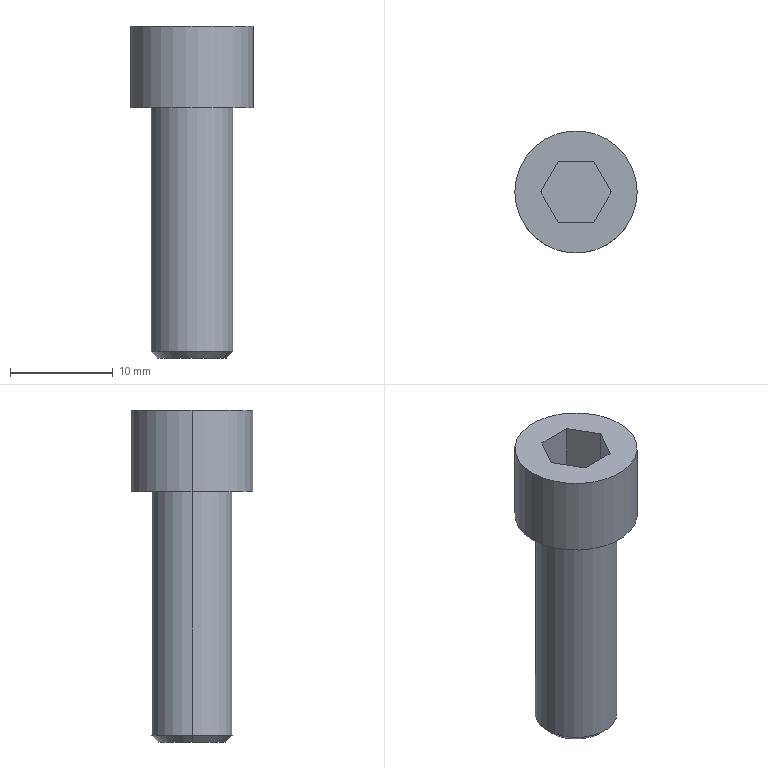Part | STEP file | 4-20.sldasm-Part-427 | 1 solid | 16 faces | box 11.91 x 11.91 x 32.34 mm | volume 1927 mm3 | plane 10 | cylinder 4 | cone 2 | commonest cylinder face diameters 7.94 x2 11.91 x2
STEP:
#1=CARTESIAN_POINT('',(-3.325,-75.,288.982));
#2=VERTEX_POINT('',#1);
#3=CARTESIAN_POINT('',(3.325,-75.,288.982));
#4=VERTEX_POINT('',#3);
#5=CARTESIAN_POINT('',(0.,-75.,288.982));
#6=DIRECTION('',(0.,0.,-1.));
#7=DIRECTION('',(1.,0.,0.));
#8=AXIS2_PLACEMENT_3D('',#5,#6,#7);
#9=CIRCLE('',#8,3.325);
#10=EDGE_CURVE('',#2,#4,#9,.T.);
#11=ORIENTED_EDGE('',*,*,#10,.F.);
#12=CARTESIAN_POINT('',(-3.97,-75.,289.627));
#13=VERTEX_POINT('',#12);
#14=CARTESIAN_POINT('',(-3.97,-75.,289.627));
#15=DIRECTION('',(-0.7071,0.,0.7071));
#16=VECTOR('',#15,1000.);
#17=LINE('',#14,#16);
#18=EDGE_CURVE('',#2,#13,#17,.T.);
#19=ORIENTED_EDGE('',*,*,#18,.T.);
#20=CARTESIAN_POINT('',(3.97,-75.,289.627));
#21=VERTEX_POINT('',#20);
#22=CARTESIAN_POINT('',(0.,-75.,289.627));
#23=DIRECTION('',(0.,0.,1.));
#24=DIRECTION('',(1.,0.,0.));
#25=AXIS2_PLACEMENT_3D('',#22,#23,#24);
#26=CIRCLE('',#25,3.97);
#27=EDGE_CURVE('',#21,#13,#26,.T.);
#28=ORIENTED_EDGE('',*,*,#27,.F.);
#29=CARTESIAN_POINT('',(3.97,-75.,289.627));
#30=DIRECTION('',(0.7071,0.,0.7071));
#31=VECTOR('',#30,1000.);
#32=LINE('',#29,#31);
#33=EDGE_CURVE('',#4,#21,#32,.T.);
#34=ORIENTED_EDGE('',*,*,#33,.F.);
#35=EDGE_LOOP('',(#11,#19,#28,#34));
#36=FACE_OUTER_BOUND('',#35,.T.);
#37=CARTESIAN_POINT('',(0.,-75.,289.627));
#38=DIRECTION('',(0.,0.,1.));
#39=DIRECTION('',(1.,0.,0.));
#40=AXIS2_PLACEMENT_3D('',#37,#38,#39);
#41=CONICAL_SURFACE('',#40,3.97,0.7854);
#42=ADVANCED_FACE('',(#36),#41,.T.);
#43=CARTESIAN_POINT('',(5.955,-75.,313.382));
#44=VERTEX_POINT('',#43);
#45=CARTESIAN_POINT('',(-5.955,-75.,313.382));
#46=VERTEX_POINT('',#45);
#47=CARTESIAN_POINT('',(0.,-75.,313.382));
#48=DIRECTION('',(0.,0.,1.));
#49=DIRECTION('',(1.,0.,0.));
#50=AXIS2_PLACEMENT_3D('',#47,#48,#49);
#51=CIRCLE('',#50,5.955);
#52=EDGE_CURVE('',#44,#46,#51,.T.);
#53=ORIENTED_EDGE('',*,*,#52,.T.);
#54=CARTESIAN_POINT('',(-5.955,-75.,321.322));
#55=VERTEX_POINT('',#54);
#56=CARTESIAN_POINT('',(-5.955,-75.,313.382));
#57=DIRECTION('',(0.,0.,1.));
#58=VECTOR('',#57,1000.);
#59=LINE('',#56,#58);
#60=EDGE_CURVE('',#46,#55,#59,.T.);
#61=ORIENTED_EDGE('',*,*,#60,.T.);
#62=CARTESIAN_POINT('',(5.955,-75.,321.322));
#63=VERTEX_POINT('',#62);
#64=CARTESIAN_POINT('',(0.,-75.,321.322));
#65=DIRECTION('',(0.,0.,1.));
#66=DIRECTION('',(1.,0.,0.));
#67=AXIS2_PLACEMENT_3D('',#64,#65,#66);
#68=CIRCLE('',#67,5.955);
#69=EDGE_CURVE('',#63,#55,#68,.T.);
#70=ORIENTED_EDGE('',*,*,#69,.F.);
#71=CARTESIAN_POINT('',(5.955,-75.,313.382));
#72=DIRECTION('',(0.,0.,1.));
#73=VECTOR('',#72,1000.);
#74=LINE('',#71,#73);
#75=EDGE_CURVE('',#44,#63,#74,.T.);
#76=ORIENTED_EDGE('',*,*,#75,.F.);
#77=EDGE_LOOP('',(#53,#61,#70,#76));
#78=FACE_OUTER_BOUND('',#77,.T.);
#79=CARTESIAN_POINT('',(0.,-75.,313.382));
#80=DIRECTION('',(0.,0.,1.));
#81=DIRECTION('',(1.,0.,0.));
#82=AXIS2_PLACEMENT_3D('',#79,#80,#81);
#83=CYLINDRICAL_SURFACE('',#82,5.955);
#84=ADVANCED_FACE('',(#78),#83,.T.);
#85=CARTESIAN_POINT('',(3.97,-75.,313.382));
#86=VERTEX_POINT('',#85);
#87=CARTESIAN_POINT('',(-3.97,-75.,313.382));
#88=VERTEX_POINT('',#87);
#89=CARTESIAN_POINT('',(0.,-75.,313.382));
#90=DIRECTION('',(0.,0.,1.));
#91=DIRECTION('',(1.,0.,0.));
#92=AXIS2_PLACEMENT_3D('',#89,#90,#91);
#93=CIRCLE('',#92,3.97);
#94=EDGE_CURVE('',#86,#88,#93,.T.);
#95=ORIENTED_EDGE('',*,*,#94,.F.);
#96=CARTESIAN_POINT('',(3.97,-75.,313.382));
#97=DIRECTION('',(0.,0.,-1.));
#98=VECTOR('',#97,1000.);
#99=LINE('',#96,#98);
#100=EDGE_CURVE('',#86,#21,#99,.T.);
#101=ORIENTED_EDGE('',*,*,#100,.T.);
#102=ORIENTED_EDGE('',*,*,#27,.T.);
#103=CARTESIAN_POINT('',(-3.97,-75.,313.382));
#104=DIRECTION('',(0.,0.,-1.));
#105=VECTOR('',#104,1000.);
#106=LINE('',#103,#105);
#107=EDGE_CURVE('',#88,#13,#106,.T.);
#108=ORIENTED_EDGE('',*,*,#107,.F.);
#109=EDGE_LOOP('',(#95,#101,#102,#108));
#110=FACE_OUTER_BOUND('',#109,.T.);
#111=CARTESIAN_POINT('',(0.,-75.,313.382));
#112=DIRECTION('',(0.,0.,-1.));
#113=DIRECTION('',(-1.,0.,0.));
#114=AXIS2_PLACEMENT_3D('',#111,#112,#113);
#115=CYLINDRICAL_SURFACE('',#114,3.97);
#116=ADVANCED_FACE('',(#110),#115,.T.);
#117=ORIENTED_EDGE('',*,*,#100,.F.);
#118=CARTESIAN_POINT('',(0.,-75.,313.382));
#119=DIRECTION('',(0.,0.,1.));
#120=DIRECTION('',(1.,0.,0.));
#121=AXIS2_PLACEMENT_3D('',#118,#119,#120);
#122=CIRCLE('',#121,3.97);
#123=EDGE_CURVE('',#88,#86,#122,.T.);
#124=ORIENTED_EDGE('',*,*,#123,.F.);
#125=ORIENTED_EDGE('',*,*,#107,.T.);
#126=CARTESIAN_POINT('',(0.,-75.,289.627));
#127=DIRECTION('',(0.,0.,1.));
#128=DIRECTION('',(1.,0.,0.));
#129=AXIS2_PLACEMENT_3D('',#126,#127,#128);
#130=CIRCLE('',#129,3.97);
#131=EDGE_CURVE('',#13,#21,#130,.T.);
#132=ORIENTED_EDGE('',*,*,#131,.T.);
#133=EDGE_LOOP('',(#117,#124,#125,#132));
#134=FACE_OUTER_BOUND('',#133,.T.);
#135=CARTESIAN_POINT('',(0.,-75.,313.382));
#136=DIRECTION('',(0.,0.,-1.));
#137=DIRECTION('',(-1.,0.,0.));
#138=AXIS2_PLACEMENT_3D('',#135,#136,#137);
#139=CYLINDRICAL_SURFACE('',#138,3.97);
#140=ADVANCED_FACE('',(#134),#139,.T.);
#141=CARTESIAN_POINT('',(0.,-75.,288.982));
#142=DIRECTION('',(0.,0.,-1.));
#143=DIRECTION('',(1.,0.,0.));
#144=AXIS2_PLACEMENT_3D('',#141,#142,#143);
#145=CIRCLE('',#144,3.325);
#146=EDGE_CURVE('',#4,#2,#145,.T.);
#147=ORIENTED_EDGE('',*,*,#146,.T.);
#148=ORIENTED_EDGE('',*,*,#10,.T.);
#149=EDGE_LOOP('',(#147,#148));
#150=FACE_OUTER_BOUND('',#149,.T.);
#151=CARTESIAN_POINT('',(0.,-75.,288.982));
#152=DIRECTION('',(0.,0.,1.));
#153=DIRECTION('',(1.,0.,0.));
#154=AXIS2_PLACEMENT_3D('',#151,#152,#153);
#155=PLANE('',#154);
#156=ADVANCED_FACE('',(#150),#155,.F.);
#157=ORIENTED_EDGE('',*,*,#52,.F.);
#158=CARTESIAN_POINT('',(0.,-75.,313.382));
#159=DIRECTION('',(0.,0.,1.));
#160=DIRECTION('',(1.,0.,0.));
#161=AXIS2_PLACEMENT_3D('',#158,#159,#160);
#162=CIRCLE('',#161,5.955);
#163=EDGE_CURVE('',#46,#44,#162,.T.);
#164=ORIENTED_EDGE('',*,*,#163,.F.);
#165=EDGE_LOOP('',(#157,#164));
#166=FACE_OUTER_BOUND('',#165,.T.);
#167=ORIENTED_EDGE('',*,*,#123,.T.);
#168=ORIENTED_EDGE('',*,*,#94,.T.);
#169=EDGE_LOOP('',(#167,#168));
#170=FACE_BOUND('',#169,.T.);
#171=CARTESIAN_POINT('',(0.,-75.,313.382));
#172=DIRECTION('',(0.,0.,-1.));
#173=DIRECTION('',(-1.,0.,0.));
#174=AXIS2_PLACEMENT_3D('',#171,#172,#173);
#175=PLANE('',#174);
#176=ADVANCED_FACE('',(#166,#170),#175,.T.);
#177=CARTESIAN_POINT('',(-1.719,-77.977,321.322));
#178=VERTEX_POINT('',#177);
#179=CARTESIAN_POINT('',(1.719,-77.977,321.322));
#180=VERTEX_POINT('',#179);
#181=CARTESIAN_POINT('',(-1.719,-77.977,321.322));
#182=DIRECTION('',(1.,0.,0.));
#183=VECTOR('',#182,1000.);
#184=LINE('',#181,#183);
#185=EDGE_CURVE('',#178,#180,#184,.T.);
#186=ORIENTED_EDGE('',*,*,#185,.F.);
#187=CARTESIAN_POINT('',(-3.438,-75.,321.322));
#188=VERTEX_POINT('',#187);
#189=CARTESIAN_POINT('',(-3.438,-75.,321.322));
#190=DIRECTION('',(0.5,-0.866,0.));
#191=VECTOR('',#190,1000.);
#192=LINE('',#189,#191);
#193=EDGE_CURVE('',#188,#178,#192,.T.);
#194=ORIENTED_EDGE('',*,*,#193,.F.);
#195=CARTESIAN_POINT('',(-1.719,-72.022,321.322));
#196=VERTEX_POINT('',#195);
#197=CARTESIAN_POINT('',(-1.719,-72.022,321.322));
#198=DIRECTION('',(-0.5,-0.866,0.));
#199=VECTOR('',#198,1000.);
#200=LINE('',#197,#199);
#201=EDGE_CURVE('',#196,#188,#200,.T.);
#202=ORIENTED_EDGE('',*,*,#201,.F.);
#203=CARTESIAN_POINT('',(1.719,-72.022,321.322));
#204=VERTEX_POINT('',#203);
#205=CARTESIAN_POINT('',(1.719,-72.022,321.322));
#206=DIRECTION('',(-1.,0.,0.));
#207=VECTOR('',#206,1000.);
#208=LINE('',#205,#207);
#209=EDGE_CURVE('',#204,#196,#208,.T.);
#210=ORIENTED_EDGE('',*,*,#209,.F.);
#211=CARTESIAN_POINT('',(3.438,-75.,321.322));
#212=VERTEX_POINT('',#211);
#213=CARTESIAN_POINT('',(3.438,-75.,321.322));
#214=DIRECTION('',(-0.5,0.866,0.));
#215=VECTOR('',#214,1000.);
#216=LINE('',#213,#215);
#217=EDGE_CURVE('',#212,#204,#216,.T.);
#218=ORIENTED_EDGE('',*,*,#217,.F.);
#219=CARTESIAN_POINT('',(1.719,-77.977,321.322));
#220=DIRECTION('',(0.5,0.866,0.));
#221=VECTOR('',#220,1000.);
#222=LINE('',#219,#221);
#223=EDGE_CURVE('',#180,#212,#222,.T.);
#224=ORIENTED_EDGE('',*,*,#223,.F.);
#225=EDGE_LOOP('',(#186,#194,#202,#210,#218,#224));
#226=FACE_BOUND('',#225,.T.);
#227=ORIENTED_EDGE('',*,*,#69,.T.);
#228=CARTESIAN_POINT('',(0.,-75.,321.322));
#229=DIRECTION('',(0.,0.,1.));
#230=DIRECTION('',(1.,0.,0.));
#231=AXIS2_PLACEMENT_3D('',#228,#229,#230);
#232=CIRCLE('',#231,5.955);
#233=EDGE_CURVE('',#55,#63,#232,.T.);
#234=ORIENTED_EDGE('',*,*,#233,.T.);
#235=EDGE_LOOP('',(#227,#234));
#236=FACE_OUTER_BOUND('',#235,.T.);
#237=CARTESIAN_POINT('',(0.,-75.,321.322));
#238=DIRECTION('',(0.,0.,1.));
#239=DIRECTION('',(1.,0.,0.));
#240=AXIS2_PLACEMENT_3D('',#237,#238,#239);
#241=PLANE('',#240);
#242=ADVANCED_FACE('',(#226,#236),#241,.T.);
#243=ORIENTED_EDGE('',*,*,#60,.F.);
#244=ORIENTED_EDGE('',*,*,#163,.T.);
#245=ORIENTED_EDGE('',*,*,#75,.T.);
#246=ORIENTED_EDGE('',*,*,#233,.F.);
#247=EDGE_LOOP('',(#243,#244,#245,#246));
#248=FACE_OUTER_BOUND('',#247,.T.);
#249=CARTESIAN_POINT('',(0.,-75.,313.382));
#250=DIRECTION('',(0.,0.,1.));
#251=DIRECTION('',(1.,0.,0.));
#252=AXIS2_PLACEMENT_3D('',#249,#250,#251);
#253=CYLINDRICAL_SURFACE('',#252,5.955);
#254=ADVANCED_FACE('',(#248),#253,.T.);
#255=ORIENTED_EDGE('',*,*,#18,.F.);
#256=ORIENTED_EDGE('',*,*,#146,.F.);
#257=ORIENTED_EDGE('',*,*,#33,.T.);
#258=ORIENTED_EDGE('',*,*,#131,.F.);
#259=EDGE_LOOP('',(#255,#256,#257,#258));
#260=FACE_OUTER_BOUND('',#259,.T.);
#261=CARTESIAN_POINT('',(0.,-75.,289.627));
#262=DIRECTION('',(0.,0.,1.));
#263=DIRECTION('',(1.,0.,0.));
#264=AXIS2_PLACEMENT_3D('',#261,#262,#263);
#265=CONICAL_SURFACE('',#264,3.97,0.7854);
#266=ADVANCED_FACE('',(#260),#265,.T.);
#267=ORIENTED_EDGE('',*,*,#185,.T.);
#268=CARTESIAN_POINT('',(1.719,-77.977,316.082));
#269=VERTEX_POINT('',#268);
#270=CARTESIAN_POINT('',(1.719,-77.977,316.082));
#271=DIRECTION('',(0.,0.,1.));
#272=VECTOR('',#271,1000.);
#273=LINE('',#270,#272);
#274=EDGE_CURVE('',#269,#180,#273,.T.);
#275=ORIENTED_EDGE('',*,*,#274,.F.);
#276=CARTESIAN_POINT('',(-1.719,-77.977,316.082));
#277=VERTEX_POINT('',#276);
#278=CARTESIAN_POINT('',(-1.719,-77.977,316.082));
#279=DIRECTION('',(1.,0.,0.));
#280=VECTOR('',#279,1000.);
#281=LINE('',#278,#280);
#282=EDGE_CURVE('',#277,#269,#281,.T.);
#283=ORIENTED_EDGE('',*,*,#282,.F.);
#284=CARTESIAN_POINT('',(-1.719,-77.977,316.082));
#285=DIRECTION('',(0.,0.,1.));
#286=VECTOR('',#285,1000.);
#287=LINE('',#284,#286);
#288=EDGE_CURVE('',#277,#178,#287,.T.);
#289=ORIENTED_EDGE('',*,*,#288,.T.);
#290=EDGE_LOOP('',(#267,#275,#283,#289));
#291=FACE_OUTER_BOUND('',#290,.T.);
#292=CARTESIAN_POINT('',(-1.719,-77.977,316.082));
#293=DIRECTION('',(0.,-1.,0.));
#294=DIRECTION('',(0.,0.,-1.));
#295=AXIS2_PLACEMENT_3D('',#292,#293,#294);
#296=PLANE('',#295);
#297=ADVANCED_FACE('',(#291),#296,.F.);
#298=ORIENTED_EDGE('',*,*,#223,.T.);
#299=CARTESIAN_POINT('',(3.438,-75.,316.082));
#300=VERTEX_POINT('',#299);
#301=CARTESIAN_POINT('',(3.438,-75.,316.082));
#302=DIRECTION('',(0.,0.,1.));
#303=VECTOR('',#302,1000.);
#304=LINE('',#301,#303);
#305=EDGE_CURVE('',#300,#212,#304,.T.);
#306=ORIENTED_EDGE('',*,*,#305,.F.);
#307=CARTESIAN_POINT('',(1.719,-77.977,316.082));
#308=DIRECTION('',(0.5,0.866,0.));
#309=VECTOR('',#308,1000.);
#310=LINE('',#307,#309);
#311=EDGE_CURVE('',#269,#300,#310,.T.);
#312=ORIENTED_EDGE('',*,*,#311,.F.);
#313=ORIENTED_EDGE('',*,*,#274,.T.);
#314=EDGE_LOOP('',(#298,#306,#312,#313));
#315=FACE_OUTER_BOUND('',#314,.T.);
#316=CARTESIAN_POINT('',(1.719,-77.977,316.082));
#317=DIRECTION('',(0.866,-0.5,0.));
#318=DIRECTION('',(0.5,0.866,0.));
#319=AXIS2_PLACEMENT_3D('',#316,#317,#318);
#320=PLANE('',#319);
#321=ADVANCED_FACE('',(#315),#320,.F.);
#322=ORIENTED_EDGE('',*,*,#217,.T.);
#323=CARTESIAN_POINT('',(1.719,-72.022,316.082));
#324=VERTEX_POINT('',#323);
#325=CARTESIAN_POINT('',(1.719,-72.022,316.082));
#326=DIRECTION('',(0.,0.,1.));
#327=VECTOR('',#326,1000.);
#328=LINE('',#325,#327);
#329=EDGE_CURVE('',#324,#204,#328,.T.);
#330=ORIENTED_EDGE('',*,*,#329,.F.);
#331=CARTESIAN_POINT('',(3.438,-75.,316.082));
#332=DIRECTION('',(-0.5,0.866,0.));
#333=VECTOR('',#332,1000.);
#334=LINE('',#331,#333);
#335=EDGE_CURVE('',#300,#324,#334,.T.);
#336=ORIENTED_EDGE('',*,*,#335,.F.);
#337=ORIENTED_EDGE('',*,*,#305,.T.);
#338=EDGE_LOOP('',(#322,#330,#336,#337));
#339=FACE_OUTER_BOUND('',#338,.T.);
#340=CARTESIAN_POINT('',(3.438,-75.,316.082));
#341=DIRECTION('',(0.866,0.5,0.));
#342=DIRECTION('',(-0.5,0.866,0.));
#343=AXIS2_PLACEMENT_3D('',#340,#341,#342);
#344=PLANE('',#343);
#345=ADVANCED_FACE('',(#339),#344,.F.);
#346=ORIENTED_EDGE('',*,*,#209,.T.);
#347=CARTESIAN_POINT('',(-1.719,-72.022,316.082));
#348=VERTEX_POINT('',#347);
#349=CARTESIAN_POINT('',(-1.719,-72.022,316.082));
#350=DIRECTION('',(0.,0.,1.));
#351=VECTOR('',#350,1000.);
#352=LINE('',#349,#351);
#353=EDGE_CURVE('',#348,#196,#352,.T.);
#354=ORIENTED_EDGE('',*,*,#353,.F.);
#355=CARTESIAN_POINT('',(1.719,-72.022,316.082));
#356=DIRECTION('',(-1.,0.,0.));
#357=VECTOR('',#356,1000.);
#358=LINE('',#355,#357);
#359=EDGE_CURVE('',#324,#348,#358,.T.);
#360=ORIENTED_EDGE('',*,*,#359,.F.);
#361=ORIENTED_EDGE('',*,*,#329,.T.);
#362=EDGE_LOOP('',(#346,#354,#360,#361));
#363=FACE_OUTER_BOUND('',#362,.T.);
#364=CARTESIAN_POINT('',(1.719,-72.022,316.082));
#365=DIRECTION('',(0.,1.,0.));
#366=DIRECTION('',(0.,0.,1.));
#367=AXIS2_PLACEMENT_3D('',#364,#365,#366);
#368=PLANE('',#367);
#369=ADVANCED_FACE('',(#363),#368,.F.);
#370=ORIENTED_EDGE('',*,*,#201,.T.);
#371=CARTESIAN_POINT('',(-3.438,-75.,316.082));
#372=VERTEX_POINT('',#371);
#373=CARTESIAN_POINT('',(-3.438,-75.,316.082));
#374=DIRECTION('',(0.,0.,1.));
#375=VECTOR('',#374,1000.);
#376=LINE('',#373,#375);
#377=EDGE_CURVE('',#372,#188,#376,.T.);
#378=ORIENTED_EDGE('',*,*,#377,.F.);
#379=CARTESIAN_POINT('',(-1.719,-72.022,316.082));
#380=DIRECTION('',(-0.5,-0.866,0.));
#381=VECTOR('',#380,1000.);
#382=LINE('',#379,#381);
#383=EDGE_CURVE('',#348,#372,#382,.T.);
#384=ORIENTED_EDGE('',*,*,#383,.F.);
#385=ORIENTED_EDGE('',*,*,#353,.T.);
#386=EDGE_LOOP('',(#370,#378,#384,#385));
#387=FACE_OUTER_BOUND('',#386,.T.);
#388=CARTESIAN_POINT('',(-1.719,-72.022,316.082));
#389=DIRECTION('',(-0.866,0.5,0.));
#390=DIRECTION('',(-0.5,-0.866,0.));
#391=AXIS2_PLACEMENT_3D('',#388,#389,#390);
#392=PLANE('',#391);
#393=ADVANCED_FACE('',(#387),#392,.F.);
#394=ORIENTED_EDGE('',*,*,#193,.T.);
#395=ORIENTED_EDGE('',*,*,#288,.F.);
#396=CARTESIAN_POINT('',(-3.438,-75.,316.082));
#397=DIRECTION('',(0.5,-0.866,0.));
#398=VECTOR('',#397,1000.);
#399=LINE('',#396,#398);
#400=EDGE_CURVE('',#372,#277,#399,.T.);
#401=ORIENTED_EDGE('',*,*,#400,.F.);
#402=ORIENTED_EDGE('',*,*,#377,.T.);
#403=EDGE_LOOP('',(#394,#395,#401,#402));
#404=FACE_OUTER_BOUND('',#403,.T.);
#405=CARTESIAN_POINT('',(-3.438,-75.,316.082));
#406=DIRECTION('',(-0.866,-0.5,0.));
#407=DIRECTION('',(0.5,-0.866,0.));
#408=AXIS2_PLACEMENT_3D('',#405,#406,#407);
#409=PLANE('',#408);
#410=ADVANCED_FACE('',(#404),#409,.F.);
#411=ORIENTED_EDGE('',*,*,#282,.T.);
#412=ORIENTED_EDGE('',*,*,#311,.T.);
#413=ORIENTED_EDGE('',*,*,#335,.T.);
#414=ORIENTED_EDGE('',*,*,#359,.T.);
#415=ORIENTED_EDGE('',*,*,#383,.T.);
#416=ORIENTED_EDGE('',*,*,#400,.T.);
#417=EDGE_LOOP('',(#411,#412,#413,#414,#415,#416));
#418=FACE_OUTER_BOUND('',#417,.T.);
#419=CARTESIAN_POINT('',(1.719,-77.977,316.082));
#420=DIRECTION('',(0.,0.,1.));
#421=DIRECTION('',(1.,0.,0.));
#422=AXIS2_PLACEMENT_3D('',#419,#420,#421);
#423=PLANE('',#422);
#424=ADVANCED_FACE('',(#418),#423,.T.);
#425=CLOSED_SHELL('',(#42,#84,#116,#140,#156,#176,#242,#254,#266,#297,#321,#345,#369,#393,#410,#424));
#426=MANIFOLD_SOLID_BREP('',#425);
#427=CARTESIAN_POINT('',(0.,0.,0.));
#428=DIRECTION('',(0.,0.,1.));
#429=DIRECTION('',(1.,0.,0.));
#430=AXIS2_PLACEMENT_3D('',#427,#428,#429);
#431=(LENGTH_UNIT()NAMED_UNIT(*)SI_UNIT(.MILLI.,.METRE.));
#432=UNCERTAINTY_MEASURE_WITH_UNIT(LENGTH_MEASURE(0.00001),#431,'','');
#433=(NAMED_UNIT(*)PLANE_ANGLE_UNIT()SI_UNIT($,.RADIAN.));
#434=(NAMED_UNIT(*)SI_UNIT($,.STERADIAN.)SOLID_ANGLE_UNIT());
#435=(GEOMETRIC_REPRESENTATION_CONTEXT(3)GLOBAL_UNCERTAINTY_ASSIGNED_CONTEXT((#432))GLOBAL_UNIT_ASSIGNED_CONTEXT((#431,#433,#434))REPRESENTATION_CONTEXT('',''));
#436=ADVANCED_BREP_SHAPE_REPRESENTATION('',(#426,#430),#435);